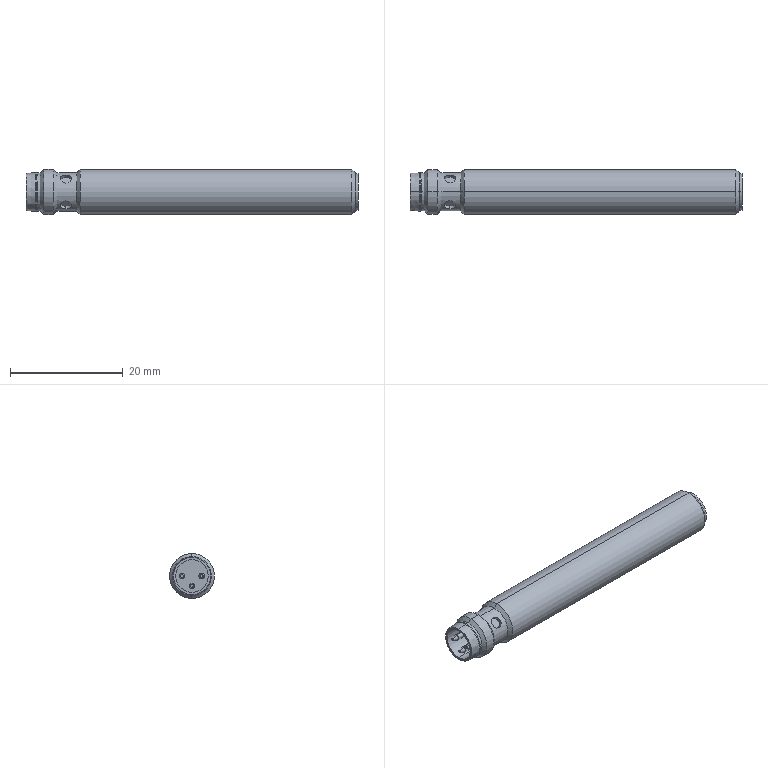Part | 1 solid | 57 faces | box 59 x 8 x 8 mm | volume 2723 mm3 | cylinder 28 | cone 18 | plane 11 | commonest cylinder face diameters 2 x8 1 x6 6.773 x4 8 x4 5.8 x2 6.5 x2